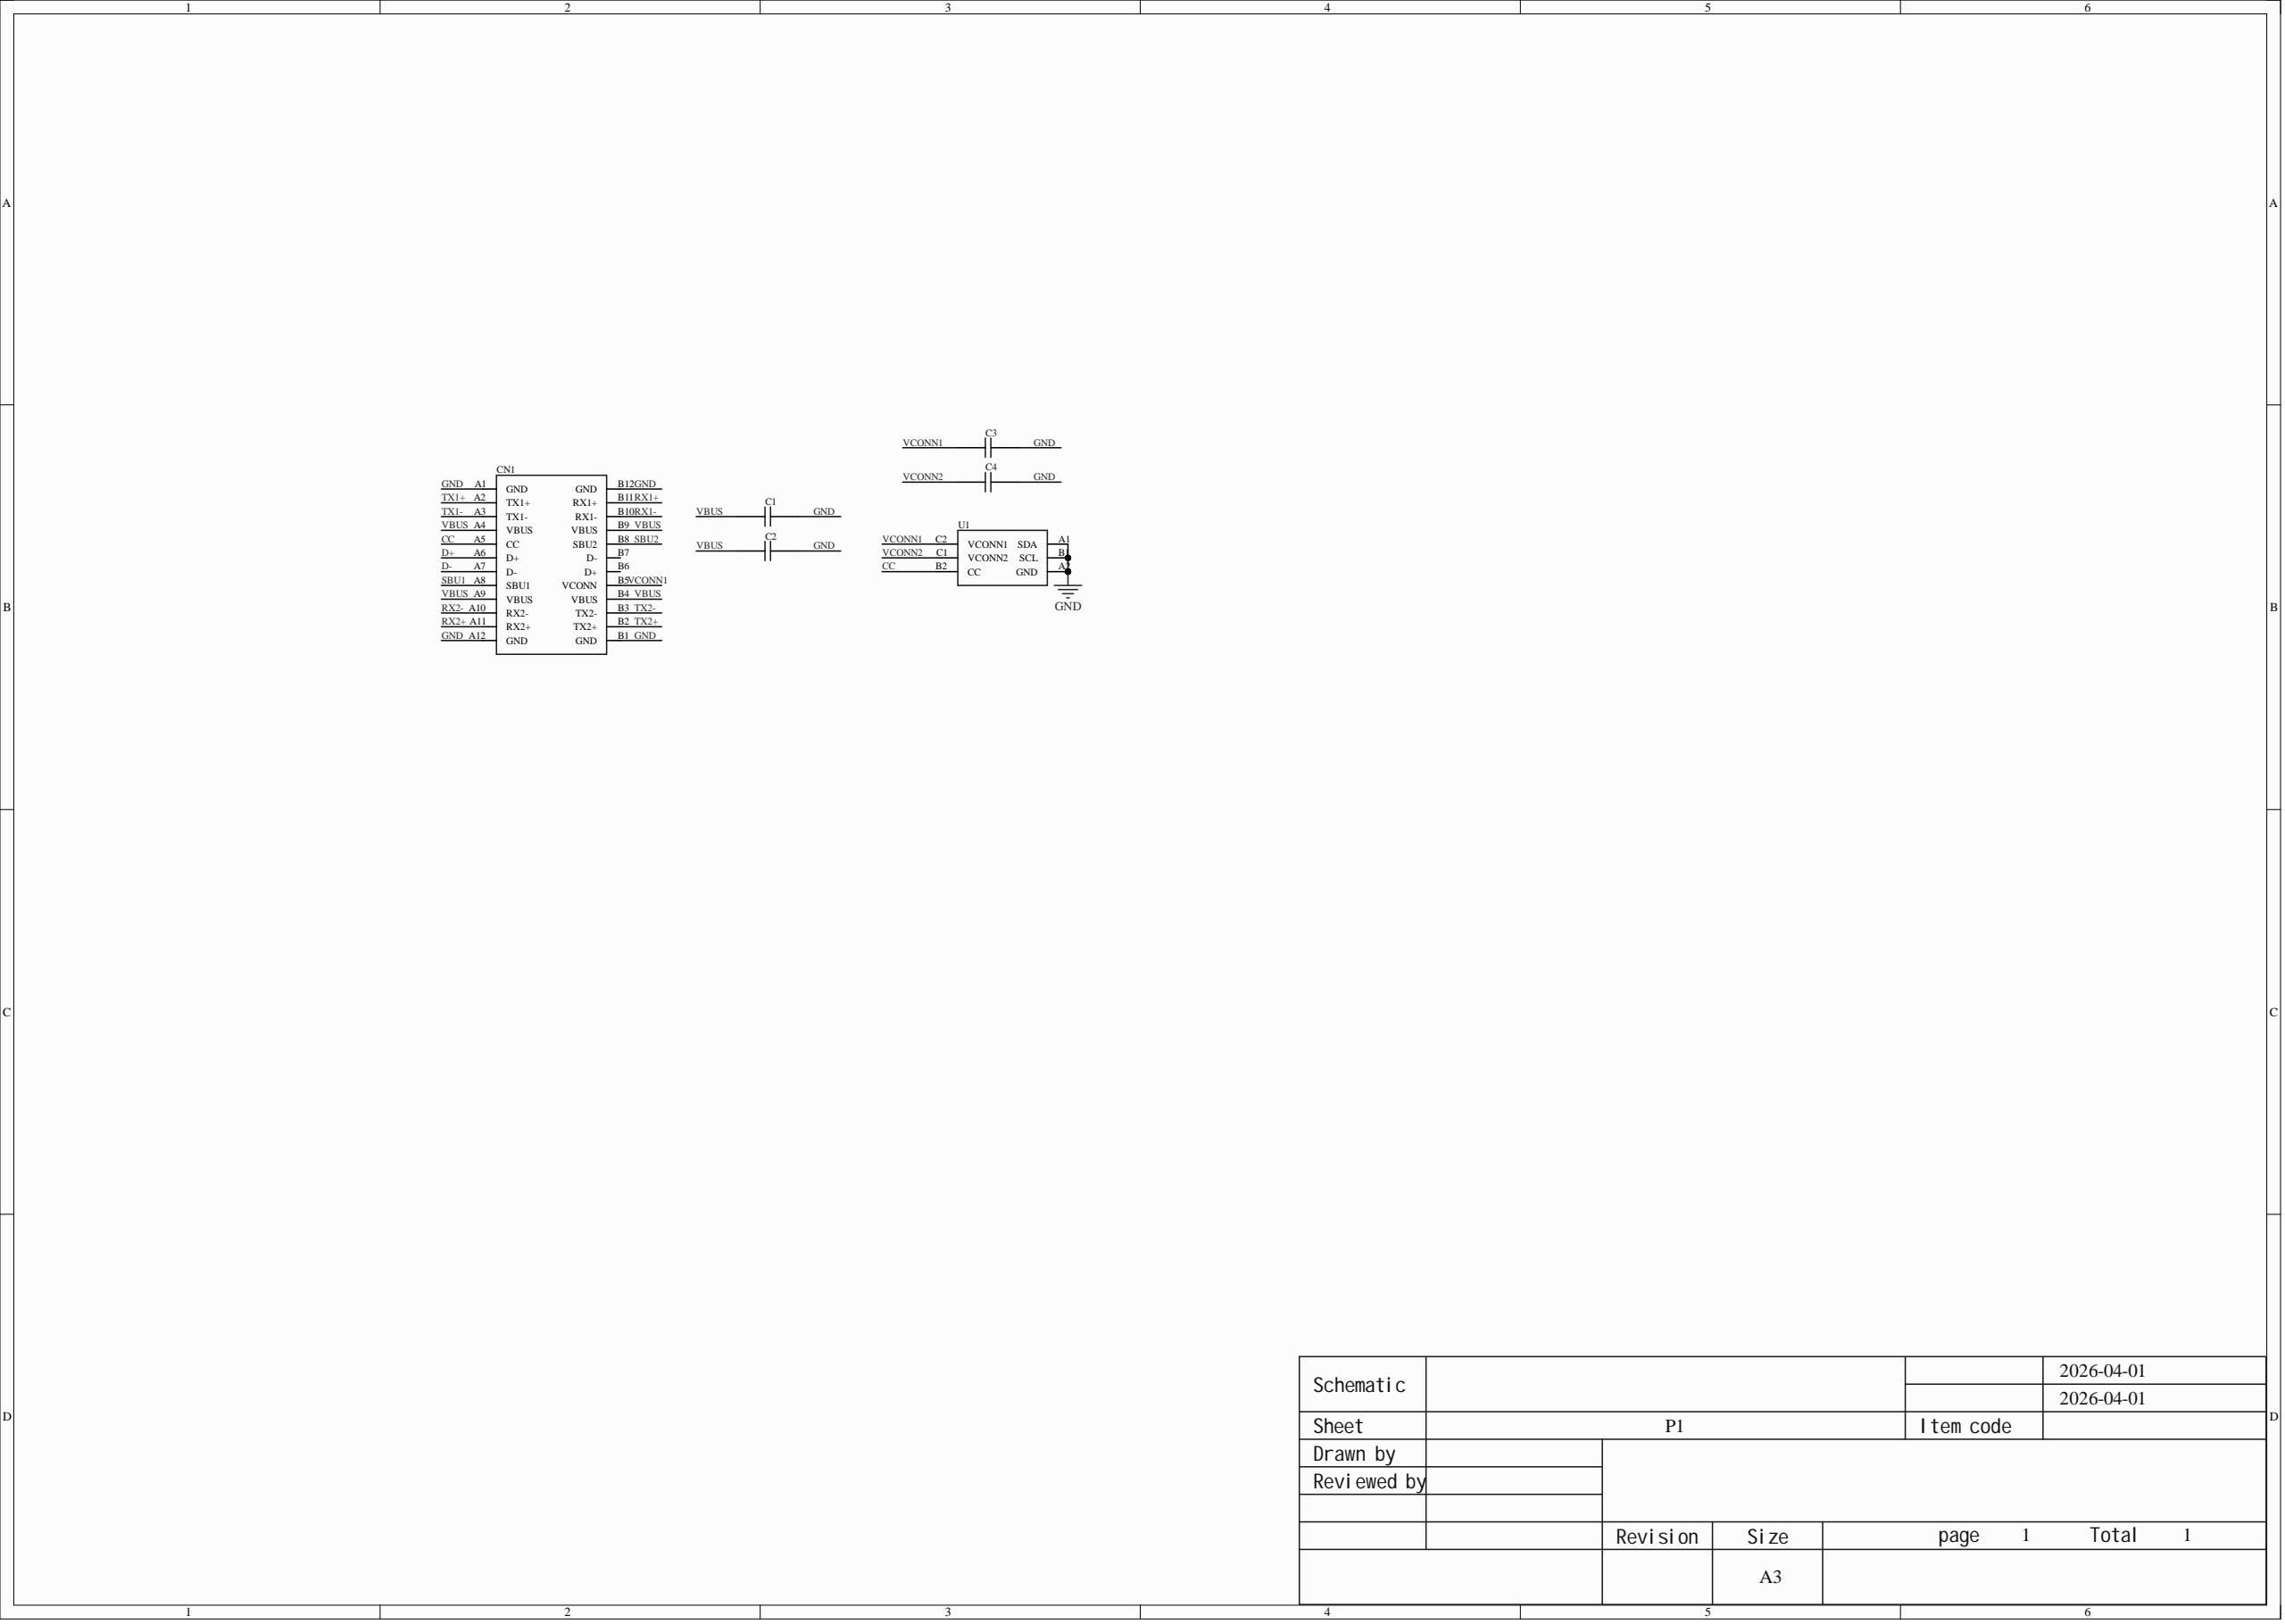Circuit board | Altium Designer | 6 parts | 5 nets
Bill of materials:
Comment,Description,Designator,Footprint,LibRef,Quantity
"GRM022R61C104ME05","","C1, C2, C3, C4","c0201","GRM022R61C104ME05","4"
"","","CN1","简易版公头","简易版公头","1"
"","","U1","wlcsp-6_l1.2-w0.8-r2-c3-p0.40-tl改","332B wlcsp-6","1"
Netlist (Protel format):
[
C1
c0201
GRM022R61C104ME05



]
[
C2
c0201
GRM022R61C104ME05



]
[
C3
c0201
GRM022R61C104ME05



]
[
C4
c0201
GRM022R61C104ME05



]
[
CN1
简易版公头




]
[
U1
wlcsp-6_l1.2-w0.8-r2-c3-p0.40-tl改




]
(
VCONN2
C4-1
U1-C1
)
(
VCONN1
C3-1
CN1-B5
U1-C2
)
(
VBUS
C1-1
C2-1
CN1-A4
CN1-A9
CN1-B4
CN1-B9
)
(
GND
C1-2
C2-2
C3-2
C4-2
CN1-A1
CN1-A12
CN1-B1
CN1-B12
U1-A1
U1-A2
U1-B1
)
(
CC
CN1-A5
U1-B2
)